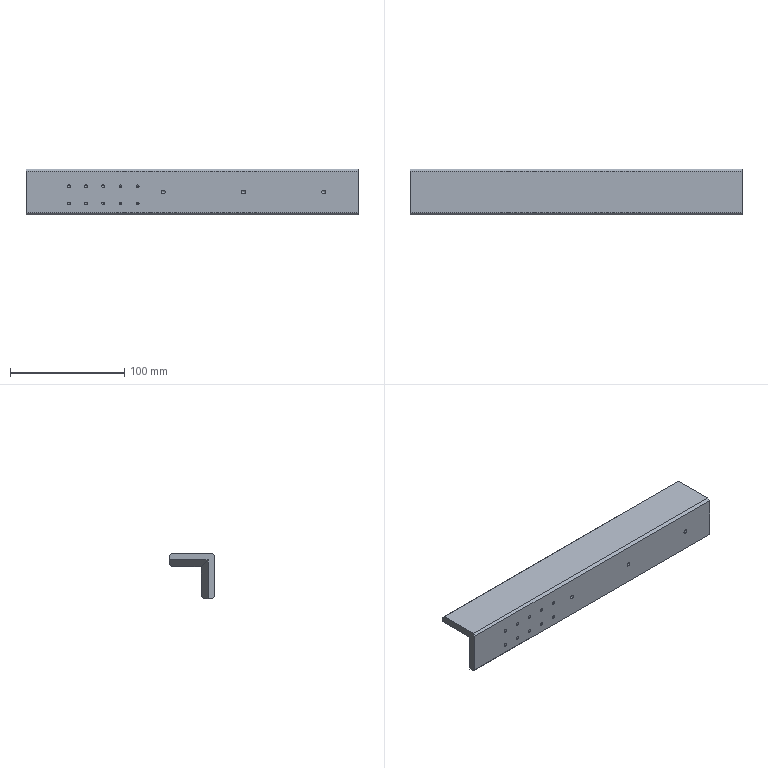Part | NX | 1 solid | 49 faces | box 290 x 40 x 40 mm | volume 230473 mm3 | cylinder 17 | cone 17 | plane 15 | commonest cylinder face diameters 2.5 x10 4.2 x4 3.3 x3
STEP:
#1=CARTESIAN_POINT('',(145.,-18.,20.));
#2=VERTEX_POINT('',#1);
#3=CARTESIAN_POINT('',(145.,-20.,18.));
#4=VERTEX_POINT('',#3);
#5=CARTESIAN_POINT('',(145.,-19.,19.));
#6=DIRECTION('',(0.,-0.7071,-0.7071));
#7=VECTOR('',#6,1000.);
#8=LINE('',#5,#7);
#9=EDGE_CURVE('',#2,#4,#8,.T.);
#10=ORIENTED_EDGE('',*,*,#9,.F.);
#11=CARTESIAN_POINT('',(-145.,-18.,20.));
#12=VERTEX_POINT('',#11);
#13=CARTESIAN_POINT('',(145.,-18.,20.));
#14=DIRECTION('',(1.,0.,0.));
#15=VECTOR('',#14,1000.);
#16=LINE('',#13,#15);
#17=EDGE_CURVE('',#12,#2,#16,.T.);
#18=ORIENTED_EDGE('',*,*,#17,.F.);
#19=CARTESIAN_POINT('',(-145.,-20.,18.));
#20=VERTEX_POINT('',#19);
#21=CARTESIAN_POINT('',(-145.,-20.,18.));
#22=DIRECTION('',(0.,0.7071,0.7071));
#23=VECTOR('',#22,1000.);
#24=LINE('',#21,#23);
#25=EDGE_CURVE('',#20,#12,#24,.T.);
#26=ORIENTED_EDGE('',*,*,#25,.F.);
#27=CARTESIAN_POINT('',(145.,-20.,18.));
#28=DIRECTION('',(-1.,0.,0.));
#29=VECTOR('',#28,1000.);
#30=LINE('',#27,#29);
#31=EDGE_CURVE('',#4,#20,#30,.T.);
#32=ORIENTED_EDGE('',*,*,#31,.F.);
#33=EDGE_LOOP('',(#10,#18,#26,#32));
#34=FACE_BOUND('',#33,.T.);
#35=CARTESIAN_POINT('',(145.,-20.,18.));
#36=DIRECTION('',(0.,0.7071,-0.7071));
#37=DIRECTION('',(-1.,0.,0.));
#38=AXIS2_PLACEMENT_3D('',#35,#36,#37);
#39=PLANE('',#38);
#40=ADVANCED_FACE('',(#34),#39,.F.);
#41=CARTESIAN_POINT('',(145.,-20.,-18.));
#42=VERTEX_POINT('',#41);
#43=CARTESIAN_POINT('',(145.,-18.,-20.));
#44=VERTEX_POINT('',#43);
#45=CARTESIAN_POINT('',(145.,-19.,-19.));
#46=DIRECTION('',(0.,0.7071,-0.7071));
#47=VECTOR('',#46,1000.);
#48=LINE('',#45,#47);
#49=EDGE_CURVE('',#42,#44,#48,.T.);
#50=ORIENTED_EDGE('',*,*,#49,.F.);
#51=CARTESIAN_POINT('',(-145.,-20.,-18.));
#52=VERTEX_POINT('',#51);
#53=CARTESIAN_POINT('',(145.,-20.,-18.));
#54=DIRECTION('',(1.,0.,0.));
#55=VECTOR('',#54,1000.);
#56=LINE('',#53,#55);
#57=EDGE_CURVE('',#52,#42,#56,.T.);
#58=ORIENTED_EDGE('',*,*,#57,.F.);
#59=CARTESIAN_POINT('',(-145.,-18.,-20.));
#60=VERTEX_POINT('',#59);
#61=CARTESIAN_POINT('',(-145.,-18.,-20.));
#62=DIRECTION('',(0.,-0.7071,0.7071));
#63=VECTOR('',#62,1000.);
#64=LINE('',#61,#63);
#65=EDGE_CURVE('',#60,#52,#64,.T.);
#66=ORIENTED_EDGE('',*,*,#65,.F.);
#67=CARTESIAN_POINT('',(145.,-18.,-20.));
#68=DIRECTION('',(-1.,0.,0.));
#69=VECTOR('',#68,1000.);
#70=LINE('',#67,#69);
#71=EDGE_CURVE('',#44,#60,#70,.T.);
#72=ORIENTED_EDGE('',*,*,#71,.F.);
#73=EDGE_LOOP('',(#50,#58,#66,#72));
#74=FACE_BOUND('',#73,.T.);
#75=CARTESIAN_POINT('',(145.,-18.,-20.));
#76=DIRECTION('',(0.,0.7071,0.7071));
#77=DIRECTION('',(-1.,0.,0.));
#78=AXIS2_PLACEMENT_3D('',#75,#76,#77);
#79=PLANE('',#78);
#80=ADVANCED_FACE('',(#74),#79,.F.);
#81=CARTESIAN_POINT('',(145.,20.,18.));
#82=VERTEX_POINT('',#81);
#83=CARTESIAN_POINT('',(145.,18.,20.));
#84=VERTEX_POINT('',#83);
#85=CARTESIAN_POINT('',(145.,19.,19.));
#86=DIRECTION('',(0.,-0.7071,0.7071));
#87=VECTOR('',#86,1000.);
#88=LINE('',#85,#87);
#89=EDGE_CURVE('',#82,#84,#88,.T.);
#90=ORIENTED_EDGE('',*,*,#89,.F.);
#91=CARTESIAN_POINT('',(-145.,20.,18.));
#92=VERTEX_POINT('',#91);
#93=CARTESIAN_POINT('',(145.,20.,18.));
#94=DIRECTION('',(1.,0.,0.));
#95=VECTOR('',#94,1000.);
#96=LINE('',#93,#95);
#97=EDGE_CURVE('',#92,#82,#96,.T.);
#98=ORIENTED_EDGE('',*,*,#97,.F.);
#99=CARTESIAN_POINT('',(-145.,18.,20.));
#100=VERTEX_POINT('',#99);
#101=CARTESIAN_POINT('',(-145.,18.,20.));
#102=DIRECTION('',(0.,0.7071,-0.7071));
#103=VECTOR('',#102,1000.);
#104=LINE('',#101,#103);
#105=EDGE_CURVE('',#100,#92,#104,.T.);
#106=ORIENTED_EDGE('',*,*,#105,.F.);
#107=CARTESIAN_POINT('',(145.,18.,20.));
#108=DIRECTION('',(-1.,0.,0.));
#109=VECTOR('',#108,1000.);
#110=LINE('',#107,#109);
#111=EDGE_CURVE('',#84,#100,#110,.T.);
#112=ORIENTED_EDGE('',*,*,#111,.F.);
#113=EDGE_LOOP('',(#90,#98,#106,#112));
#114=FACE_BOUND('',#113,.T.);
#115=CARTESIAN_POINT('',(145.,18.,20.));
#116=DIRECTION('',(0.,-0.7071,-0.7071));
#117=DIRECTION('',(-1.,0.,0.));
#118=AXIS2_PLACEMENT_3D('',#115,#116,#117);
#119=PLANE('',#118);
#120=ADVANCED_FACE('',(#114),#119,.F.);
#121=CARTESIAN_POINT('',(-138.333,20.,10.));
#122=VERTEX_POINT('',#121);
#123=CARTESIAN_POINT('',(-135.,18.,8.));
#124=VERTEX_POINT('',#123);
#125=CARTESIAN_POINT('',(-136.628,18.977,8.977));
#126=DIRECTION('',(0.7625,-0.4575,-0.4575));
#127=VECTOR('',#126,1000.);
#128=LINE('',#125,#127);
#129=EDGE_CURVE('',#122,#124,#128,.T.);
#130=ORIENTED_EDGE('',*,*,#129,.F.);
#131=CARTESIAN_POINT('',(145.,20.,10.));
#132=VERTEX_POINT('',#131);
#133=CARTESIAN_POINT('',(145.,20.,10.));
#134=DIRECTION('',(-1.,0.,0.));
#135=VECTOR('',#134,1000.);
#136=LINE('',#133,#135);
#137=EDGE_CURVE('',#132,#122,#136,.T.);
#138=ORIENTED_EDGE('',*,*,#137,.F.);
#139=CARTESIAN_POINT('',(145.,18.,8.));
#140=VERTEX_POINT('',#139);
#141=CARTESIAN_POINT('',(145.,5.,-5.));
#142=DIRECTION('',(0.,0.7071,0.7071));
#143=VECTOR('',#142,1000.);
#144=LINE('',#141,#143);
#145=EDGE_CURVE('',#140,#132,#144,.T.);
#146=ORIENTED_EDGE('',*,*,#145,.F.);
#147=CARTESIAN_POINT('',(-145.,18.,8.));
#148=DIRECTION('',(1.,0.,0.));
#149=VECTOR('',#148,1000.);
#150=LINE('',#147,#149);
#151=EDGE_CURVE('',#124,#140,#150,.T.);
#152=ORIENTED_EDGE('',*,*,#151,.F.);
#153=EDGE_LOOP('',(#130,#138,#146,#152));
#154=FACE_BOUND('',#153,.T.);
#155=CARTESIAN_POINT('',(145.,-10.,-20.));
#156=DIRECTION('',(0.,-0.7071,0.7071));
#157=DIRECTION('',(1.,0.,0.));
#158=AXIS2_PLACEMENT_3D('',#155,#156,#157);
#159=PLANE('',#158);
#160=ADVANCED_FACE('',(#154),#159,.F.);
#161=CARTESIAN_POINT('',(-135.,-8.,-18.));
#162=VERTEX_POINT('',#161);
#163=CARTESIAN_POINT('',(-138.333,-10.,-20.));
#164=VERTEX_POINT('',#163);
#165=CARTESIAN_POINT('',(-136.628,-8.977,-18.977));
#166=DIRECTION('',(-0.7625,-0.4575,-0.4575));
#167=VECTOR('',#166,1000.);
#168=LINE('',#165,#167);
#169=EDGE_CURVE('',#162,#164,#168,.T.);
#170=ORIENTED_EDGE('',*,*,#169,.F.);
#171=CARTESIAN_POINT('',(145.,-8.,-18.));
#172=VERTEX_POINT('',#171);
#173=CARTESIAN_POINT('',(-145.,-8.,-18.));
#174=DIRECTION('',(-1.,0.,0.));
#175=VECTOR('',#174,1000.);
#176=LINE('',#173,#175);
#177=EDGE_CURVE('',#172,#162,#176,.T.);
#178=ORIENTED_EDGE('',*,*,#177,.F.);
#179=CARTESIAN_POINT('',(145.,-10.,-20.));
#180=VERTEX_POINT('',#179);
#181=CARTESIAN_POINT('',(145.,5.,-5.));
#182=DIRECTION('',(0.,0.7071,0.7071));
#183=VECTOR('',#182,1000.);
#184=LINE('',#181,#183);
#185=EDGE_CURVE('',#180,#172,#184,.T.);
#186=ORIENTED_EDGE('',*,*,#185,.F.);
#187=CARTESIAN_POINT('',(145.,-10.,-20.));
#188=DIRECTION('',(1.,0.,0.));
#189=VECTOR('',#188,1000.);
#190=LINE('',#187,#189);
#191=EDGE_CURVE('',#164,#180,#190,.T.);
#192=ORIENTED_EDGE('',*,*,#191,.F.);
#193=EDGE_LOOP('',(#170,#178,#186,#192));
#194=FACE_BOUND('',#193,.T.);
#195=CARTESIAN_POINT('',(145.,-10.,-20.));
#196=DIRECTION('',(0.,-0.7071,0.7071));
#197=DIRECTION('',(1.,0.,0.));
#198=AXIS2_PLACEMENT_3D('',#195,#196,#197);
#199=PLANE('',#198);
#200=ADVANCED_FACE('',(#194),#199,.F.);
#201=CARTESIAN_POINT('',(-135.,-8.,8.));
#202=VERTEX_POINT('',#201);
#203=CARTESIAN_POINT('',(-135.,-8.,-20.));
#204=DIRECTION('',(0.,0.,1.));
#205=VECTOR('',#204,1000.);
#206=LINE('',#203,#205);
#207=EDGE_CURVE('',#162,#202,#206,.T.);
#208=ORIENTED_EDGE('',*,*,#207,.F.);
#209=ORIENTED_EDGE('',*,*,#169,.T.);
#210=CARTESIAN_POINT('',(-145.,-14.,-20.));
#211=VERTEX_POINT('',#210);
#212=CARTESIAN_POINT('',(-145.,-14.,-20.));
#213=DIRECTION('',(0.8575,0.5145,0.));
#214=VECTOR('',#213,1000.);
#215=LINE('',#212,#214);
#216=EDGE_CURVE('',#211,#164,#215,.T.);
#217=ORIENTED_EDGE('',*,*,#216,.F.);
#218=CARTESIAN_POINT('',(-145.,-14.,14.));
#219=VERTEX_POINT('',#218);
#220=CARTESIAN_POINT('',(-145.,-14.,0.));
#221=DIRECTION('',(0.,0.,-1.));
#222=VECTOR('',#221,1000.);
#223=LINE('',#220,#222);
#224=EDGE_CURVE('',#219,#211,#223,.T.);
#225=ORIENTED_EDGE('',*,*,#224,.F.);
#226=CARTESIAN_POINT('',(-140.116,-11.07,11.07));
#227=DIRECTION('',(0.7625,0.4575,-0.4575));
#228=VECTOR('',#227,1000.);
#229=LINE('',#226,#228);
#230=EDGE_CURVE('',#219,#202,#229,.T.);
#231=ORIENTED_EDGE('',*,*,#230,.T.);
#232=EDGE_LOOP('',(#208,#209,#217,#225,#231));
#233=FACE_BOUND('',#232,.T.);
#234=CARTESIAN_POINT('',(-145.,-14.,0.));
#235=DIRECTION('',(0.5145,-0.8575,0.));
#236=DIRECTION('',(0.,0.,-1.));
#237=AXIS2_PLACEMENT_3D('',#234,#235,#236);
#238=PLANE('',#237);
#239=ADVANCED_FACE('',(#233),#238,.F.);
#240=CARTESIAN_POINT('',(-145.,20.,14.));
#241=VERTEX_POINT('',#240);
#242=CARTESIAN_POINT('',(-145.,20.,14.));
#243=DIRECTION('',(-0.8575,0.,0.5145));
#244=VECTOR('',#243,1000.);
#245=LINE('',#242,#244);
#246=EDGE_CURVE('',#122,#241,#245,.T.);
#247=ORIENTED_EDGE('',*,*,#246,.F.);
#248=ORIENTED_EDGE('',*,*,#129,.T.);
#249=CARTESIAN_POINT('',(-135.,20.,8.));
#250=DIRECTION('',(0.,1.,0.));
#251=VECTOR('',#250,1000.);
#252=LINE('',#249,#251);
#253=EDGE_CURVE('',#202,#124,#252,.T.);
#254=ORIENTED_EDGE('',*,*,#253,.F.);
#255=ORIENTED_EDGE('',*,*,#230,.F.);
#256=CARTESIAN_POINT('',(-145.,0.,14.));
#257=DIRECTION('',(0.,-1.,0.));
#258=VECTOR('',#257,1000.);
#259=LINE('',#256,#258);
#260=EDGE_CURVE('',#241,#219,#259,.T.);
#261=ORIENTED_EDGE('',*,*,#260,.F.);
#262=EDGE_LOOP('',(#247,#248,#254,#255,#261));
#263=FACE_BOUND('',#262,.T.);
#264=CARTESIAN_POINT('',(-145.,0.,14.));
#265=DIRECTION('',(0.5145,0.,0.8575));
#266=DIRECTION('',(0.,-1.,0.));
#267=AXIS2_PLACEMENT_3D('',#264,#265,#266);
#268=PLANE('',#267);
#269=ADVANCED_FACE('',(#263),#268,.F.);
#270=ORIENTED_EDGE('',*,*,#253,.T.);
#271=ORIENTED_EDGE('',*,*,#151,.T.);
#272=CARTESIAN_POINT('',(145.,-8.,8.));
#273=VERTEX_POINT('',#272);
#274=CARTESIAN_POINT('',(145.,20.,8.));
#275=DIRECTION('',(0.,-1.,0.));
#276=VECTOR('',#275,1000.);
#277=LINE('',#274,#276);
#278=EDGE_CURVE('',#140,#273,#277,.T.);
#279=ORIENTED_EDGE('',*,*,#278,.T.);
#280=CARTESIAN_POINT('',(-145.,-8.,8.));
#281=DIRECTION('',(1.,0.,0.));
#282=VECTOR('',#281,1000.);
#283=LINE('',#280,#282);
#284=EDGE_CURVE('',#202,#273,#283,.T.);
#285=ORIENTED_EDGE('',*,*,#284,.F.);
#286=EDGE_LOOP('',(#270,#271,#279,#285));
#287=FACE_BOUND('',#286,.T.);
#288=CARTESIAN_POINT('',(-145.,20.,8.));
#289=DIRECTION('',(0.,0.,1.));
#290=DIRECTION('',(0.,-1.,0.));
#291=AXIS2_PLACEMENT_3D('',#288,#289,#290);
#292=PLANE('',#291);
#293=ADVANCED_FACE('',(#287),#292,.F.);
#294=CARTESIAN_POINT('',(145.,-8.,-20.));
#295=DIRECTION('',(0.,0.,-1.));
#296=VECTOR('',#295,1000.);
#297=LINE('',#294,#296);
#298=EDGE_CURVE('',#273,#172,#297,.T.);
#299=ORIENTED_EDGE('',*,*,#298,.T.);
#300=ORIENTED_EDGE('',*,*,#177,.T.);
#301=ORIENTED_EDGE('',*,*,#207,.T.);
#302=ORIENTED_EDGE('',*,*,#284,.T.);
#303=EDGE_LOOP('',(#299,#300,#301,#302));
#304=FACE_BOUND('',#303,.T.);
#305=CARTESIAN_POINT('',(-145.,-8.,-20.));
#306=DIRECTION('',(0.,-1.,0.));
#307=DIRECTION('',(0.,0.,-1.));
#308=AXIS2_PLACEMENT_3D('',#305,#306,#307);
#309=PLANE('',#308);
#310=ADVANCED_FACE('',(#304),#309,.F.);
#311=CARTESIAN_POINT('',(-145.,20.,20.));
#312=DIRECTION('',(0.,-1.,0.));
#313=VECTOR('',#312,1000.);
#314=LINE('',#311,#313);
#315=EDGE_CURVE('',#100,#12,#314,.T.);
#316=ORIENTED_EDGE('',*,*,#315,.F.);
#317=ORIENTED_EDGE('',*,*,#105,.T.);
#318=CARTESIAN_POINT('',(-145.,20.,20.));
#319=DIRECTION('',(0.,0.,1.));
#320=VECTOR('',#319,1000.);
#321=LINE('',#318,#320);
#322=EDGE_CURVE('',#241,#92,#321,.T.);
#323=ORIENTED_EDGE('',*,*,#322,.F.);
#324=ORIENTED_EDGE('',*,*,#260,.T.);
#325=ORIENTED_EDGE('',*,*,#224,.T.);
#326=CARTESIAN_POINT('',(-145.,20.,-20.));
#327=DIRECTION('',(0.,1.,0.));
#328=VECTOR('',#327,1000.);
#329=LINE('',#326,#328);
#330=EDGE_CURVE('',#60,#211,#329,.T.);
#331=ORIENTED_EDGE('',*,*,#330,.F.);
#332=ORIENTED_EDGE('',*,*,#65,.T.);
#333=CARTESIAN_POINT('',(-145.,-20.,20.));
#334=DIRECTION('',(0.,0.,-1.));
#335=VECTOR('',#334,1000.);
#336=LINE('',#333,#335);
#337=EDGE_CURVE('',#20,#52,#336,.T.);
#338=ORIENTED_EDGE('',*,*,#337,.F.);
#339=ORIENTED_EDGE('',*,*,#25,.T.);
#340=EDGE_LOOP('',(#316,#317,#323,#324,#325,#331,#332,#338,#339));
#341=FACE_BOUND('',#340,.T.);
#342=CARTESIAN_POINT('',(-145.,0.,0.));
#343=DIRECTION('',(1.,0.,0.));
#344=DIRECTION('',(0.,0.,-1.));
#345=AXIS2_PLACEMENT_3D('',#342,#343,#344);
#346=PLANE('',#345);
#347=ADVANCED_FACE('',(#341),#346,.F.);
#348=CARTESIAN_POINT('',(145.,20.,-20.));
#349=DIRECTION('',(0.,1.,0.));
#350=VECTOR('',#349,1000.);
#351=LINE('',#348,#350);
#352=EDGE_CURVE('',#44,#180,#351,.T.);
#353=ORIENTED_EDGE('',*,*,#352,.T.);
#354=ORIENTED_EDGE('',*,*,#185,.T.);
#355=ORIENTED_EDGE('',*,*,#298,.F.);
#356=ORIENTED_EDGE('',*,*,#278,.F.);
#357=ORIENTED_EDGE('',*,*,#145,.T.);
#358=CARTESIAN_POINT('',(145.,20.,20.));
#359=DIRECTION('',(0.,0.,1.));
#360=VECTOR('',#359,1000.);
#361=LINE('',#358,#360);
#362=EDGE_CURVE('',#132,#82,#361,.T.);
#363=ORIENTED_EDGE('',*,*,#362,.T.);
#364=ORIENTED_EDGE('',*,*,#89,.T.);
#365=CARTESIAN_POINT('',(145.,20.,20.));
#366=DIRECTION('',(0.,-1.,0.));
#367=VECTOR('',#366,1000.);
#368=LINE('',#365,#367);
#369=EDGE_CURVE('',#84,#2,#368,.T.);
#370=ORIENTED_EDGE('',*,*,#369,.T.);
#371=ORIENTED_EDGE('',*,*,#9,.T.);
#372=CARTESIAN_POINT('',(145.,-20.,20.));
#373=DIRECTION('',(0.,0.,-1.));
#374=VECTOR('',#373,1000.);
#375=LINE('',#372,#374);
#376=EDGE_CURVE('',#4,#42,#375,.T.);
#377=ORIENTED_EDGE('',*,*,#376,.T.);
#378=ORIENTED_EDGE('',*,*,#49,.T.);
#379=EDGE_LOOP('',(#353,#354,#355,#356,#357,#363,#364,#370,#371,#377,#378));
#380=FACE_BOUND('',#379,.T.);
#381=CARTESIAN_POINT('',(145.,14.,11.9));
#382=VERTEX_POINT('',#381);
#383=CARTESIAN_POINT('',(145.,14.,14.));
#384=DIRECTION('',(1.,0.,0.));
#385=DIRECTION('',(0.,0.,-1.));
#386=AXIS2_PLACEMENT_3D('',#383,#384,#385);
#387=CIRCLE('',#386,2.1);
#388=EDGE_CURVE('',#382,#382,#387,.T.);
#389=ORIENTED_EDGE('',*,*,#388,.F.);
#390=EDGE_LOOP('',(#389));
#391=FACE_BOUND('',#390,.T.);
#392=CARTESIAN_POINT('',(145.,-2.,11.9));
#393=VERTEX_POINT('',#392);
#394=CARTESIAN_POINT('',(145.,-2.,14.));
#395=DIRECTION('',(1.,0.,0.));
#396=DIRECTION('',(0.,0.,-1.));
#397=AXIS2_PLACEMENT_3D('',#394,#395,#396);
#398=CIRCLE('',#397,2.1);
#399=EDGE_CURVE('',#393,#393,#398,.T.);
#400=ORIENTED_EDGE('',*,*,#399,.F.);
#401=EDGE_LOOP('',(#400));
#402=FACE_BOUND('',#401,.T.);
#403=CARTESIAN_POINT('',(145.,-14.,-0.1));
#404=VERTEX_POINT('',#403);
#405=CARTESIAN_POINT('',(145.,-14.,2.));
#406=DIRECTION('',(1.,0.,0.));
#407=DIRECTION('',(0.,0.,-1.));
#408=AXIS2_PLACEMENT_3D('',#405,#406,#407);
#409=CIRCLE('',#408,2.1);
#410=EDGE_CURVE('',#404,#404,#409,.T.);
#411=ORIENTED_EDGE('',*,*,#410,.F.);
#412=EDGE_LOOP('',(#411));
#413=FACE_BOUND('',#412,.T.);
#414=CARTESIAN_POINT('',(145.,-14.,-16.1));
#415=VERTEX_POINT('',#414);
#416=CARTESIAN_POINT('',(145.,-14.,-14.));
#417=DIRECTION('',(1.,0.,0.));
#418=DIRECTION('',(0.,0.,-1.));
#419=AXIS2_PLACEMENT_3D('',#416,#417,#418);
#420=CIRCLE('',#419,2.1);
#421=EDGE_CURVE('',#415,#415,#420,.T.);
#422=ORIENTED_EDGE('',*,*,#421,.F.);
#423=EDGE_LOOP('',(#422));
#424=FACE_BOUND('',#423,.T.);
#425=CARTESIAN_POINT('',(145.,0.,0.));
#426=DIRECTION('',(1.,0.,0.));
#427=DIRECTION('',(0.,0.,-1.));
#428=AXIS2_PLACEMENT_3D('',#425,#426,#427);
#429=PLANE('',#428);
#430=ADVANCED_FACE('',(#380,#391,#402,#413,#424),#429,.T.);
#431=CARTESIAN_POINT('',(-107.5,-20.,3.75));
#432=VERTEX_POINT('',#431);
#433=CARTESIAN_POINT('',(-107.5,-20.,5.));
#434=DIRECTION('',(0.,-1.,0.));
#435=DIRECTION('',(0.,0.,-1.));
#436=AXIS2_PLACEMENT_3D('',#433,#434,#435);
#437=CIRCLE('',#436,1.25);
#438=EDGE_CURVE('',#432,#432,#437,.T.);
#439=ORIENTED_EDGE('',*,*,#438,.F.);
#440=EDGE_LOOP('',(#439));
#441=FACE_BOUND('',#440,.T.);
#442=CARTESIAN_POINT('',(-92.5,-20.,3.75));
#443=VERTEX_POINT('',#442);
#444=CARTESIAN_POINT('',(-92.5,-20.,5.));
#445=DIRECTION('',(0.,-1.,0.));
#446=DIRECTION('',(0.,0.,-1.));
#447=AXIS2_PLACEMENT_3D('',#444,#445,#446);
#448=CIRCLE('',#447,1.25);
#449=EDGE_CURVE('',#443,#443,#448,.T.);
#450=ORIENTED_EDGE('',*,*,#449,.F.);
#451=EDGE_LOOP('',(#450));
#452=FACE_BOUND('',#451,.T.);
#453=CARTESIAN_POINT('',(-77.5,-20.,3.75));
#454=VERTEX_POINT('',#453);
#455=CARTESIAN_POINT('',(-77.5,-20.,5.));
#456=DIRECTION('',(0.,-1.,0.));
#457=DIRECTION('',(0.,0.,-1.));
#458=AXIS2_PLACEMENT_3D('',#455,#456,#457);
#459=CIRCLE('',#458,1.25);
#460=EDGE_CURVE('',#454,#454,#459,.T.);
#461=ORIENTED_EDGE('',*,*,#460,.F.);
#462=EDGE_LOOP('',(#461));
#463=FACE_BOUND('',#462,.T.);
#464=CARTESIAN_POINT('',(-107.5,-20.,-11.25));
#465=VERTEX_POINT('',#464);
#466=CARTESIAN_POINT('',(-107.5,-20.,-10.));
#467=DIRECTION('',(0.,-1.,0.));
#468=DIRECTION('',(0.,0.,-1.));
#469=AXIS2_PLACEMENT_3D('',#466,#467,#468);
#470=CIRCLE('',#469,1.25);
#471=EDGE_CURVE('',#465,#465,#470,.T.);
#472=ORIENTED_EDGE('',*,*,#471,.F.);
#473=EDGE_LOOP('',(#472));
#474=FACE_BOUND('',#473,.T.);
#475=CARTESIAN_POINT('',(-92.5,-20.,-11.25));
#476=VERTEX_POINT('',#475);
#477=CARTESIAN_POINT('',(-92.5,-20.,-10.));
#478=DIRECTION('',(0.,-1.,0.));
#479=DIRECTION('',(0.,0.,-1.));
#480=AXIS2_PLACEMENT_3D('',#477,#478,#479);
#481=CIRCLE('',#480,1.25);
#482=EDGE_CURVE('',#476,#476,#481,.T.);
#483=ORIENTED_EDGE('',*,*,#482,.F.);
#484=EDGE_LOOP('',(#483));
#485=FACE_BOUND('',#484,.T.);
#486=CARTESIAN_POINT('',(-77.5,-20.,-11.25));
#487=VERTEX_POINT('',#486);
#488=CARTESIAN_POINT('',(-77.5,-20.,-10.));
#489=DIRECTION('',(0.,-1.,0.));
#490=DIRECTION('',(0.,0.,-1.));
#491=AXIS2_PLACEMENT_3D('',#488,#489,#490);
#492=CIRCLE('',#491,1.25);
#493=EDGE_CURVE('',#487,#487,#492,.T.);
#494=ORIENTED_EDGE('',*,*,#493,.F.);
#495=EDGE_LOOP('',(#494));
#496=FACE_BOUND('',#495,.T.);
#497=ORIENTED_EDGE('',*,*,#337,.T.);
#498=ORIENTED_EDGE('',*,*,#57,.T.);
#499=ORIENTED_EDGE('',*,*,#376,.F.);
#500=ORIENTED_EDGE('',*,*,#31,.T.);
#501=EDGE_LOOP('',(#497,#498,#499,#500));
#502=FACE_BOUND('',#501,.T.);
#503=CARTESIAN_POINT('',(-47.5,-20.,3.75));
#504=VERTEX_POINT('',#503);
#505=CARTESIAN_POINT('',(-47.5,-20.,5.));
#506=DIRECTION('',(0.,-1.,0.));
#507=DIRECTION('',(0.,0.,-1.));
#508=AXIS2_PLACEMENT_3D('',#505,#506,#507);
#509=CIRCLE('',#508,1.25);
#510=EDGE_CURVE('',#504,#504,#509,.T.);
#511=ORIENTED_EDGE('',*,*,#510,.F.);
#512=EDGE_LOOP('',(#511));
#513=FACE_BOUND('',#512,.T.);
#514=CARTESIAN_POINT('',(-47.5,-20.,-11.25));
#515=VERTEX_POINT('',#514);
#516=CARTESIAN_POINT('',(-47.5,-20.,-10.));
#517=DIRECTION('',(0.,-1.,0.));
#518=DIRECTION('',(0.,0.,-1.));
#519=AXIS2_PLACEMENT_3D('',#516,#517,#518);
#520=CIRCLE('',#519,1.25);
#521=EDGE_CURVE('',#515,#515,#520,.T.);
#522=ORIENTED_EDGE('',*,*,#521,.F.);
#523=EDGE_LOOP('',(#522));
#524=FACE_BOUND('',#523,.T.);
#525=CARTESIAN_POINT('',(-62.5,-20.,-11.25));
#526=VERTEX_POINT('',#525);
#527=CARTESIAN_POINT('',(-62.5,-20.,-10.));
#528=DIRECTION('',(0.,-1.,0.));
#529=DIRECTION('',(0.,0.,-1.));
#530=AXIS2_PLACEMENT_3D('',#527,#528,#529);
#531=CIRCLE('',#530,1.25);
#532=EDGE_CURVE('',#526,#526,#531,.T.);
#533=ORIENTED_EDGE('',*,*,#532,.F.);
#534=EDGE_LOOP('',(#533));
#535=FACE_BOUND('',#534,.T.);
#536=CARTESIAN_POINT('',(-62.5,-20.,3.75));
#537=VERTEX_POINT('',#536);
#538=CARTESIAN_POINT('',(-62.5,-20.,5.));
#539=DIRECTION('',(0.,-1.,0.));
#540=DIRECTION('',(0.,0.,-1.));
#541=AXIS2_PLACEMENT_3D('',#538,#539,#540);
#542=CIRCLE('',#541,1.25);
#543=EDGE_CURVE('',#537,#537,#542,.T.);
#544=ORIENTED_EDGE('',*,*,#543,.F.);
#545=EDGE_LOOP('',(#544));
#546=FACE_BOUND('',#545,.T.);
#547=CARTESIAN_POINT('',(115.,-20.,-1.65));
#548=VERTEX_POINT('',#547);
#549=CARTESIAN_POINT('',(115.,-20.,0.));
#550=DIRECTION('',(0.,-1.,0.));
#551=DIRECTION('',(0.,0.,-1.));
#552=AXIS2_PLACEMENT_3D('',#549,#550,#551);
#553=CIRCLE('',#552,1.65);
#554=EDGE_CURVE('',#548,#548,#553,.T.);
#555=ORIENTED_EDGE('',*,*,#554,.F.);
#556=EDGE_LOOP('',(#555));
#557=FACE_BOUND('',#556,.T.);
#558=CARTESIAN_POINT('',(45.,-20.,-1.65));
#559=VERTEX_POINT('',#558);
#560=CARTESIAN_POINT('',(45.,-20.,0.));
#561=DIRECTION('',(0.,-1.,0.));
#562=DIRECTION('',(0.,0.,-1.));
#563=AXIS2_PLACEMENT_3D('',#560,#561,#562);
#564=CIRCLE('',#563,1.65);
#565=EDGE_CURVE('',#559,#559,#564,.T.);
#566=ORIENTED_EDGE('',*,*,#565,.F.);
#567=EDGE_LOOP('',(#566));
#568=FACE_BOUND('',#567,.T.);
#569=CARTESIAN_POINT('',(-25.,-20.,-1.65));
#570=VERTEX_POINT('',#569);
#571=CARTESIAN_POINT('',(-25.,-20.,0.));
#572=DIRECTION('',(0.,-1.,0.));
#573=DIRECTION('',(0.,0.,-1.));
#574=AXIS2_PLACEMENT_3D('',#571,#572,#573);
#575=CIRCLE('',#574,1.65);
#576=EDGE_CURVE('',#570,#570,#575,.T.);
#577=ORIENTED_EDGE('',*,*,#576,.F.);
#578=EDGE_LOOP('',(#577));
#579=FACE_BOUND('',#578,.T.);
#580=CARTESIAN_POINT('',(145.,-20.,20.));
#581=DIRECTION('',(0.,1.,0.));
#582=DIRECTION('',(0.,0.,1.));
#583=AXIS2_PLACEMENT_3D('',#580,#581,#582);
#584=PLANE('',#583);
#585=ADVANCED_FACE('',(#441,#452,#463,#474,#485,#496,#502,#513,#524,#535,#546,#557,#568,#579),#584,.F.);
#586=ORIENTED_EDGE('',*,*,#369,.F.);
#587=ORIENTED_EDGE('',*,*,#111,.T.);
#588=ORIENTED_EDGE('',*,*,#315,.T.);
#589=ORIENTED_EDGE('',*,*,#17,.T.);
#590=EDGE_LOOP('',(#586,#587,#588,#589));
#591=FACE_BOUND('',#590,.T.);
#592=CARTESIAN_POINT('',(145.,20.,20.));
#593=DIRECTION('',(0.,0.,-1.));
#594=DIRECTION('',(0.,1.,0.));
#595=AXIS2_PLACEMENT_3D('',#592,#593,#594);
#596=PLANE('',#595);
#597=ADVANCED_FACE('',(#591),#596,.F.);
#598=ORIENTED_EDGE('',*,*,#362,.F.);
#599=ORIENTED_EDGE('',*,*,#137,.T.);
#600=ORIENTED_EDGE('',*,*,#246,.T.);
#601=ORIENTED_EDGE('',*,*,#322,.T.);
#602=ORIENTED_EDGE('',*,*,#97,.T.);
#603=EDGE_LOOP('',(#598,#599,#600,#601,#602));
#604=FACE_BOUND('',#603,.T.);
#605=CARTESIAN_POINT('',(145.,20.,20.));
#606=DIRECTION('',(0.,-1.,0.));
#607=DIRECTION('',(0.,0.,-1.));
#608=AXIS2_PLACEMENT_3D('',#605,#606,#607);
#609=PLANE('',#608);
#610=ADVANCED_FACE('',(#604),#609,.F.);
#611=ORIENTED_EDGE('',*,*,#216,.T.);
#612=ORIENTED_EDGE('',*,*,#191,.T.);
#613=ORIENTED_EDGE('',*,*,#352,.F.);
#614=ORIENTED_EDGE('',*,*,#71,.T.);
#615=ORIENTED_EDGE('',*,*,#330,.T.);
#616=EDGE_LOOP('',(#611,#612,#613,#614,#615));
#617=FACE_BOUND('',#616,.T.);
#618=CARTESIAN_POINT('',(145.,20.,-20.));
#619=DIRECTION('',(0.,0.,1.));
#620=DIRECTION('',(0.,-1.,0.));
#621=AXIS2_PLACEMENT_3D('',#618,#619,#620);
#622=PLANE('',#621);
#623=ADVANCED_FACE('',(#617),#622,.F.);
#624=ORIENTED_EDGE('',*,*,#438,.T.);
#625=EDGE_LOOP('',(#624));
#626=FACE_BOUND('',#625,.T.);
#627=CARTESIAN_POINT('',(-107.5,-12.5,3.75));
#628=VERTEX_POINT('',#627);
#629=CARTESIAN_POINT('',(-107.5,-12.5,5.));
#630=DIRECTION('',(0.,-1.,0.));
#631=DIRECTION('',(0.,0.,-1.));
#632=AXIS2_PLACEMENT_3D('',#629,#630,#631);
#633=CIRCLE('',#632,1.25);
#634=EDGE_CURVE('',#628,#628,#633,.T.);
#635=ORIENTED_EDGE('',*,*,#634,.F.);
#636=EDGE_LOOP('',(#635));
#637=FACE_BOUND('',#636,.T.);
#638=CARTESIAN_POINT('',(-107.5,-20.,5.));
#639=DIRECTION('',(0.,-1.,0.));
#640=DIRECTION('',(0.,0.,-1.));
#641=AXIS2_PLACEMENT_3D('',#638,#639,#640);
#642=CYLINDRICAL_SURFACE('',#641,1.25);
#643=ADVANCED_FACE('',(#626,#637),#642,.F.);
#644=CARTESIAN_POINT('',(-107.5,-11.749,5.));
#645=VERTEX_POINT('',#644);
#646=VERTEX_LOOP('',#645);
#647=FACE_BOUND('',#646,.T.);
#648=ORIENTED_EDGE('',*,*,#634,.T.);
#649=EDGE_LOOP('',(#648));
#650=FACE_BOUND('',#649,.T.);
#651=CARTESIAN_POINT('',(-107.5,-12.5,5.));
#652=DIRECTION('',(0.,-1.,0.));
#653=DIRECTION('',(0.,0.,-1.));
#654=AXIS2_PLACEMENT_3D('',#651,#652,#653);
#655=CONICAL_SURFACE('',#654,1.25,1.03);
#656=ADVANCED_FACE('',(#647,#650),#655,.F.);
#657=ORIENTED_EDGE('',*,*,#449,.T.);
#658=EDGE_LOOP('',(#657));
#659=FACE_BOUND('',#658,.T.);
#660=CARTESIAN_POINT('',(-92.5,-12.5,3.75));
#661=VERTEX_POINT('',#660);
#662=CARTESIAN_POINT('',(-92.5,-12.5,5.));
#663=DIRECTION('',(0.,-1.,0.));
#664=DIRECTION('',(0.,0.,-1.));
#665=AXIS2_PLACEMENT_3D('',#662,#663,#664);
#666=CIRCLE('',#665,1.25);
#667=EDGE_CURVE('',#661,#661,#666,.T.);
#668=ORIENTED_EDGE('',*,*,#667,.F.);
#669=EDGE_LOOP('',(#668));
#670=FACE_BOUND('',#669,.T.);
#671=CARTESIAN_POINT('',(-92.5,-20.,5.));
#672=DIRECTION('',(0.,-1.,0.));
#673=DIRECTION('',(0.,0.,-1.));
#674=AXIS2_PLACEMENT_3D('',#671,#672,#673);
#675=CYLINDRICAL_SURFACE('',#674,1.25);
#676=ADVANCED_FACE('',(#659,#670),#675,.F.);
#677=CARTESIAN_POINT('',(-92.5,-11.749,5.));
#678=VERTEX_POINT('',#677);
#679=VERTEX_LOOP('',#678);
#680=FACE_BOUND('',#679,.T.);
#681=ORIENTED_EDGE('',*,*,#667,.T.);
#682=EDGE_LOOP('',(#681));
#683=FACE_BOUND('',#682,.T.);
#684=CARTESIAN_POINT('',(-92.5,-12.5,5.));
#685=DIRECTION('',(0.,-1.,0.));
#686=DIRECTION('',(0.,0.,-1.));
#687=AXIS2_PLACEMENT_3D('',#684,#685,#686);
#688=CONICAL_SURFACE('',#687,1.25,1.03);
#689=ADVANCED_FACE('',(#680,#683),#688,.F.);
#690=ORIENTED_EDGE('',*,*,#460,.T.);
#691=EDGE_LOOP('',(#690));
#692=FACE_BOUND('',#691,.T.);
#693=CARTESIAN_POINT('',(-77.5,-12.5,3.75));
#694=VERTEX_POINT('',#693);
#695=CARTESIAN_POINT('',(-77.5,-12.5,5.));
#696=DIRECTION('',(0.,-1.,0.));
#697=DIRECTION('',(0.,0.,-1.));
#698=AXIS2_PLACEMENT_3D('',#695,#696,#697);
#699=CIRCLE('',#698,1.25);
#700=EDGE_CURVE('',#694,#694,#699,.T.);
#701=ORIENTED_EDGE('',*,*,#700,.F.);
#702=EDGE_LOOP('',(#701));
#703=FACE_BOUND('',#702,.T.);
#704=CARTESIAN_POINT('',(-77.5,-20.,5.));
#705=DIRECTION('',(0.,-1.,0.));
#706=DIRECTION('',(0.,0.,-1.));
#707=AXIS2_PLACEMENT_3D('',#704,#705,#706);
#708=CYLINDRICAL_SURFACE('',#707,1.25);
#709=ADVANCED_FACE('',(#692,#703),#708,.F.);
#710=CARTESIAN_POINT('',(-77.5,-11.749,5.));
#711=VERTEX_POINT('',#710);
#712=VERTEX_LOOP('',#711);
#713=FACE_BOUND('',#712,.T.);
#714=ORIENTED_EDGE('',*,*,#700,.T.);
#715=EDGE_LOOP('',(#714));
#716=FACE_BOUND('',#715,.T.);
#717=CARTESIAN_POINT('',(-77.5,-12.5,5.));
#718=DIRECTION('',(0.,-1.,0.));
#719=DIRECTION('',(0.,0.,-1.));
#720=AXIS2_PLACEMENT_3D('',#717,#718,#719);
#721=CONICAL_SURFACE('',#720,1.25,1.03);
#722=ADVANCED_FACE('',(#713,#716),#721,.F.);
#723=ORIENTED_EDGE('',*,*,#471,.T.);
#724=EDGE_LOOP('',(#723));
#725=FACE_BOUND('',#724,.T.);
#726=CARTESIAN_POINT('',(-107.5,-12.5,-11.25));
#727=VERTEX_POINT('',#726);
#728=CARTESIAN_POINT('',(-107.5,-12.5,-10.));
#729=DIRECTION('',(0.,-1.,0.));
#730=DIRECTION('',(0.,0.,-1.));
#731=AXIS2_PLACEMENT_3D('',#728,#729,#730);
#732=CIRCLE('',#731,1.25);
#733=EDGE_CURVE('',#727,#727,#732,.T.);
#734=ORIENTED_EDGE('',*,*,#733,.F.);
#735=EDGE_LOOP('',(#734));
#736=FACE_BOUND('',#735,.T.);
#737=CARTESIAN_POINT('',(-107.5,-20.,-10.));
#738=DIRECTION('',(0.,-1.,0.));
#739=DIRECTION('',(0.,0.,-1.));
#740=AXIS2_PLACEMENT_3D('',#737,#738,#739);
#741=CYLINDRICAL_SURFACE('',#740,1.25);
#742=ADVANCED_FACE('',(#725,#736),#741,.F.);
#743=CARTESIAN_POINT('',(-107.5,-11.749,-10.));
#744=VERTEX_POINT('',#743);
#745=VERTEX_LOOP('',#744);
#746=FACE_BOUND('',#745,.T.);
#747=ORIENTED_EDGE('',*,*,#733,.T.);
#748=EDGE_LOOP('',(#747));
#749=FACE_BOUND('',#748,.T.);
#750=CARTESIAN_POINT('',(-107.5,-12.5,-10.));
#751=DIRECTION('',(0.,-1.,0.));
#752=DIRECTION('',(0.,0.,-1.));
#753=AXIS2_PLACEMENT_3D('',#750,#751,#752);
#754=CONICAL_SURFACE('',#753,1.25,1.03);
#755=ADVANCED_FACE('',(#746,#749),#754,.F.);
#756=ORIENTED_EDGE('',*,*,#482,.T.);
#757=EDGE_LOOP('',(#756));
#758=FACE_BOUND('',#757,.T.);
#759=CARTESIAN_POINT('',(-92.5,-12.5,-11.25));
#760=VERTEX_POINT('',#759);
#761=CARTESIAN_POINT('',(-92.5,-12.5,-10.));
#762=DIRECTION('',(0.,-1.,0.));
#763=DIRECTION('',(0.,0.,-1.));
#764=AXIS2_PLACEMENT_3D('',#761,#762,#763);
#765=CIRCLE('',#764,1.25);
#766=EDGE_CURVE('',#760,#760,#765,.T.);
#767=ORIENTED_EDGE('',*,*,#766,.F.);
#768=EDGE_LOOP('',(#767));
#769=FACE_BOUND('',#768,.T.);
#770=CARTESIAN_POINT('',(-92.5,-20.,-10.));
#771=DIRECTION('',(0.,-1.,0.));
#772=DIRECTION('',(0.,0.,-1.));
#773=AXIS2_PLACEMENT_3D('',#770,#771,#772);
#774=CYLINDRICAL_SURFACE('',#773,1.25);
#775=ADVANCED_FACE('',(#758,#769),#774,.F.);
#776=CARTESIAN_POINT('',(-92.5,-11.749,-10.));
#777=VERTEX_POINT('',#776);
#778=VERTEX_LOOP('',#777);
#779=FACE_BOUND('',#778,.T.);
#780=ORIENTED_EDGE('',*,*,#766,.T.);
#781=EDGE_LOOP('',(#780));
#782=FACE_BOUND('',#781,.T.);
#783=CARTESIAN_POINT('',(-92.5,-12.5,-10.));
#784=DIRECTION('',(0.,-1.,0.));
#785=DIRECTION('',(0.,0.,-1.));
#786=AXIS2_PLACEMENT_3D('',#783,#784,#785);
#787=CONICAL_SURFACE('',#786,1.25,1.03);
#788=ADVANCED_FACE('',(#779,#782),#787,.F.);
#789=ORIENTED_EDGE('',*,*,#493,.T.);
#790=EDGE_LOOP('',(#789));
#791=FACE_BOUND('',#790,.T.);
#792=CARTESIAN_POINT('',(-77.5,-12.5,-11.25));
#793=VERTEX_POINT('',#792);
#794=CARTESIAN_POINT('',(-77.5,-12.5,-10.));
#795=DIRECTION('',(0.,-1.,0.));
#796=DIRECTION('',(0.,0.,-1.));
#797=AXIS2_PLACEMENT_3D('',#794,#795,#796);
#798=CIRCLE('',#797,1.25);
#799=EDGE_CURVE('',#793,#793,#798,.T.);
#800=ORIENTED_EDGE('',*,*,#799,.F.);
#801=EDGE_LOOP('',(#800));
#802=FACE_BOUND('',#801,.T.);
#803=CARTESIAN_POINT('',(-77.5,-20.,-10.));
#804=DIRECTION('',(0.,-1.,0.));
#805=DIRECTION('',(0.,0.,-1.));
#806=AXIS2_PLACEMENT_3D('',#803,#804,#805);
#807=CYLINDRICAL_SURFACE('',#806,1.25);
#808=ADVANCED_FACE('',(#791,#802),#807,.F.);
#809=CARTESIAN_POINT('',(-77.5,-11.749,-10.));
#810=VERTEX_POINT('',#809);
#811=VERTEX_LOOP('',#810);
#812=FACE_BOUND('',#811,.T.);
#813=ORIENTED_EDGE('',*,*,#799,.T.);
#814=EDGE_LOOP('',(#813));
#815=FACE_BOUND('',#814,.T.);
#816=CARTESIAN_POINT('',(-77.5,-12.5,-10.));
#817=DIRECTION('',(0.,-1.,0.));
#818=DIRECTION('',(0.,0.,-1.));
#819=AXIS2_PLACEMENT_3D('',#816,#817,#818);
#820=CONICAL_SURFACE('',#819,1.25,1.03);
#821=ADVANCED_FACE('',(#812,#815),#820,.F.);
#822=CARTESIAN_POINT('',(128.738,14.,14.));
#823=VERTEX_POINT('',#822);
#824=VERTEX_LOOP('',#823);
#825=FACE_BOUND('',#824,.T.);
#826=CARTESIAN_POINT('',(130.,14.,11.9));
#827=VERTEX_POINT('',#826);
#828=CARTESIAN_POINT('',(130.,14.,14.));
#829=DIRECTION('',(1.,0.,0.));
#830=DIRECTION('',(0.,0.,-1.));
#831=AXIS2_PLACEMENT_3D('',#828,#829,#830);
#832=CIRCLE('',#831,2.1);
#833=EDGE_CURVE('',#827,#827,#832,.T.);
#834=ORIENTED_EDGE('',*,*,#833,.T.);
#835=EDGE_LOOP('',(#834));
#836=FACE_BOUND('',#835,.T.);
#837=CARTESIAN_POINT('',(130.,14.,14.));
#838=DIRECTION('',(1.,0.,0.));
#839=DIRECTION('',(0.,0.,-1.));
#840=AXIS2_PLACEMENT_3D('',#837,#838,#839);
#841=CONICAL_SURFACE('',#840,2.1,1.03);
#842=ADVANCED_FACE('',(#825,#836),#841,.F.);
#843=ORIENTED_EDGE('',*,*,#388,.T.);
#844=EDGE_LOOP('',(#843));
#845=FACE_BOUND('',#844,.T.);
#846=ORIENTED_EDGE('',*,*,#833,.F.);
#847=EDGE_LOOP('',(#846));
#848=FACE_BOUND('',#847,.T.);
#849=CARTESIAN_POINT('',(145.,14.,14.));
#850=DIRECTION('',(1.,0.,0.));
#851=DIRECTION('',(0.,0.,-1.));
#852=AXIS2_PLACEMENT_3D('',#849,#850,#851);
#853=CYLINDRICAL_SURFACE('',#852,2.1);
#854=ADVANCED_FACE('',(#845,#848),#853,.F.);
#855=CARTESIAN_POINT('',(128.738,-2.,14.));
#856=VERTEX_POINT('',#855);
#857=VERTEX_LOOP('',#856);
#858=FACE_BOUND('',#857,.T.);
#859=CARTESIAN_POINT('',(130.,-2.,11.9));
#860=VERTEX_POINT('',#859);
#861=CARTESIAN_POINT('',(130.,-2.,14.));
#862=DIRECTION('',(1.,0.,0.));
#863=DIRECTION('',(0.,0.,-1.));
#864=AXIS2_PLACEMENT_3D('',#861,#862,#863);
#865=CIRCLE('',#864,2.1);
#866=EDGE_CURVE('',#860,#860,#865,.T.);
#867=ORIENTED_EDGE('',*,*,#866,.T.);
#868=EDGE_LOOP('',(#867));
#869=FACE_BOUND('',#868,.T.);
#870=CARTESIAN_POINT('',(130.,-2.,14.));
#871=DIRECTION('',(1.,0.,0.));
#872=DIRECTION('',(0.,0.,-1.));
#873=AXIS2_PLACEMENT_3D('',#870,#871,#872);
#874=CONICAL_SURFACE('',#873,2.1,1.03);
#875=ADVANCED_FACE('',(#858,#869),#874,.F.);
#876=ORIENTED_EDGE('',*,*,#399,.T.);
#877=EDGE_LOOP('',(#876));
#878=FACE_BOUND('',#877,.T.);
#879=ORIENTED_EDGE('',*,*,#866,.F.);
#880=EDGE_LOOP('',(#879));
#881=FACE_BOUND('',#880,.T.);
#882=CARTESIAN_POINT('',(145.,-2.,14.));
#883=DIRECTION('',(1.,0.,0.));
#884=DIRECTION('',(0.,0.,-1.));
#885=AXIS2_PLACEMENT_3D('',#882,#883,#884);
#886=CYLINDRICAL_SURFACE('',#885,2.1);
#887=ADVANCED_FACE('',(#878,#881),#886,.F.);
#888=CARTESIAN_POINT('',(128.738,-14.,2.));
#889=VERTEX_POINT('',#888);
#890=VERTEX_LOOP('',#889);
#891=FACE_BOUND('',#890,.T.);
#892=CARTESIAN_POINT('',(130.,-14.,-0.1));
#893=VERTEX_POINT('',#892);
#894=CARTESIAN_POINT('',(130.,-14.,2.));
#895=DIRECTION('',(1.,0.,0.));
#896=DIRECTION('',(0.,0.,-1.));
#897=AXIS2_PLACEMENT_3D('',#894,#895,#896);
#898=CIRCLE('',#897,2.1);
#899=EDGE_CURVE('',#893,#893,#898,.T.);
#900=ORIENTED_EDGE('',*,*,#899,.T.);
#901=EDGE_LOOP('',(#900));
#902=FACE_BOUND('',#901,.T.);
#903=CARTESIAN_POINT('',(130.,-14.,2.));
#904=DIRECTION('',(1.,0.,0.));
#905=DIRECTION('',(0.,0.,-1.));
#906=AXIS2_PLACEMENT_3D('',#903,#904,#905);
#907=CONICAL_SURFACE('',#906,2.1,1.03);
#908=ADVANCED_FACE('',(#891,#902),#907,.F.);
#909=ORIENTED_EDGE('',*,*,#410,.T.);
#910=EDGE_LOOP('',(#909));
#911=FACE_BOUND('',#910,.T.);
#912=ORIENTED_EDGE('',*,*,#899,.F.);
#913=EDGE_LOOP('',(#912));
#914=FACE_BOUND('',#913,.T.);
#915=CARTESIAN_POINT('',(145.,-14.,2.));
#916=DIRECTION('',(1.,0.,0.));
#917=DIRECTION('',(0.,0.,-1.));
#918=AXIS2_PLACEMENT_3D('',#915,#916,#917);
#919=CYLINDRICAL_SURFACE('',#918,2.1);
#920=ADVANCED_FACE('',(#911,#914),#919,.F.);
#921=CARTESIAN_POINT('',(128.738,-14.,-14.));
#922=VERTEX_POINT('',#921);
#923=VERTEX_LOOP('',#922);
#924=FACE_BOUND('',#923,.T.);
#925=CARTESIAN_POINT('',(130.,-14.,-16.1));
#926=VERTEX_POINT('',#925);
#927=CARTESIAN_POINT('',(130.,-14.,-14.));
#928=DIRECTION('',(1.,0.,0.));
#929=DIRECTION('',(0.,0.,-1.));
#930=AXIS2_PLACEMENT_3D('',#927,#928,#929);
#931=CIRCLE('',#930,2.1);
#932=EDGE_CURVE('',#926,#926,#931,.T.);
#933=ORIENTED_EDGE('',*,*,#932,.T.);
#934=EDGE_LOOP('',(#933));
#935=FACE_BOUND('',#934,.T.);
#936=CARTESIAN_POINT('',(130.,-14.,-14.));
#937=DIRECTION('',(1.,0.,0.));
#938=DIRECTION('',(0.,0.,-1.));
#939=AXIS2_PLACEMENT_3D('',#936,#937,#938);
#940=CONICAL_SURFACE('',#939,2.1,1.03);
#941=ADVANCED_FACE('',(#924,#935),#940,.F.);
#942=ORIENTED_EDGE('',*,*,#421,.T.);
#943=EDGE_LOOP('',(#942));
#944=FACE_BOUND('',#943,.T.);
#945=ORIENTED_EDGE('',*,*,#932,.F.);
#946=EDGE_LOOP('',(#945));
#947=FACE_BOUND('',#946,.T.);
#948=CARTESIAN_POINT('',(145.,-14.,-14.));
#949=DIRECTION('',(1.,0.,0.));
#950=DIRECTION('',(0.,0.,-1.));
#951=AXIS2_PLACEMENT_3D('',#948,#949,#950);
#952=CYLINDRICAL_SURFACE('',#951,2.1);
#953=ADVANCED_FACE('',(#944,#947),#952,.F.);
#954=CARTESIAN_POINT('',(-47.5,-11.749,5.));
#955=VERTEX_POINT('',#954);
#956=VERTEX_LOOP('',#955);
#957=FACE_BOUND('',#956,.T.);
#958=CARTESIAN_POINT('',(-47.5,-12.5,3.75));
#959=VERTEX_POINT('',#958);
#960=CARTESIAN_POINT('',(-47.5,-12.5,5.));
#961=DIRECTION('',(0.,-1.,0.));
#962=DIRECTION('',(0.,0.,-1.));
#963=AXIS2_PLACEMENT_3D('',#960,#961,#962);
#964=CIRCLE('',#963,1.25);
#965=EDGE_CURVE('',#959,#959,#964,.T.);
#966=ORIENTED_EDGE('',*,*,#965,.T.);
#967=EDGE_LOOP('',(#966));
#968=FACE_BOUND('',#967,.T.);
#969=CARTESIAN_POINT('',(-47.5,-12.5,5.));
#970=DIRECTION('',(0.,-1.,0.));
#971=DIRECTION('',(0.,0.,-1.));
#972=AXIS2_PLACEMENT_3D('',#969,#970,#971);
#973=CONICAL_SURFACE('',#972,1.25,1.03);
#974=ADVANCED_FACE('',(#957,#968),#973,.F.);
#975=ORIENTED_EDGE('',*,*,#510,.T.);
#976=EDGE_LOOP('',(#975));
#977=FACE_BOUND('',#976,.T.);
#978=ORIENTED_EDGE('',*,*,#965,.F.);
#979=EDGE_LOOP('',(#978));
#980=FACE_BOUND('',#979,.T.);
#981=CARTESIAN_POINT('',(-47.5,-20.,5.));
#982=DIRECTION('',(0.,-1.,0.));
#983=DIRECTION('',(0.,0.,-1.));
#984=AXIS2_PLACEMENT_3D('',#981,#982,#983);
#985=CYLINDRICAL_SURFACE('',#984,1.25);
#986=ADVANCED_FACE('',(#977,#980),#985,.F.);
#987=CARTESIAN_POINT('',(-47.5,-11.749,-10.));
#988=VERTEX_POINT('',#987);
#989=VERTEX_LOOP('',#988);
#990=FACE_BOUND('',#989,.T.);
#991=CARTESIAN_POINT('',(-47.5,-12.5,-11.25));
#992=VERTEX_POINT('',#991);
#993=CARTESIAN_POINT('',(-47.5,-12.5,-10.));
#994=DIRECTION('',(0.,-1.,0.));
#995=DIRECTION('',(0.,0.,-1.));
#996=AXIS2_PLACEMENT_3D('',#993,#994,#995);
#997=CIRCLE('',#996,1.25);
#998=EDGE_CURVE('',#992,#992,#997,.T.);
#999=ORIENTED_EDGE('',*,*,#998,.T.);
#1000=EDGE_LOOP('',(#999));
#1001=FACE_BOUND('',#1000,.T.);
#1002=CARTESIAN_POINT('',(-47.5,-12.5,-10.));
#1003=DIRECTION('',(0.,-1.,0.));
#1004=DIRECTION('',(0.,0.,-1.));
#1005=AXIS2_PLACEMENT_3D('',#1002,#1003,#1004);
#1006=CONICAL_SURFACE('',#1005,1.25,1.03);
#1007=ADVANCED_FACE('',(#990,#1001),#1006,.F.);
#1008=ORIENTED_EDGE('',*,*,#521,.T.);
#1009=EDGE_LOOP('',(#1008));
#1010=FACE_BOUND('',#1009,.T.);
#1011=ORIENTED_EDGE('',*,*,#998,.F.);
#1012=EDGE_LOOP('',(#1011));
#1013=FACE_BOUND('',#1012,.T.);
#1014=CARTESIAN_POINT('',(-47.5,-20.,-10.));
#1015=DIRECTION('',(0.,-1.,0.));
#1016=DIRECTION('',(0.,0.,-1.));
#1017=AXIS2_PLACEMENT_3D('',#1014,#1015,#1016);
#1018=CYLINDRICAL_SURFACE('',#1017,1.25);
#1019=ADVANCED_FACE('',(#1010,#1013),#1018,.F.);
#1020=CARTESIAN_POINT('',(-62.5,-11.749,-10.));
#1021=VERTEX_POINT('',#1020);
#1022=VERTEX_LOOP('',#1021);
#1023=FACE_BOUND('',#1022,.T.);
#1024=CARTESIAN_POINT('',(-62.5,-12.5,-11.25));
#1025=VERTEX_POINT('',#1024);
#1026=CARTESIAN_POINT('',(-62.5,-12.5,-10.));
#1027=DIRECTION('',(0.,-1.,0.));
#1028=DIRECTION('',(0.,0.,-1.));
#1029=AXIS2_PLACEMENT_3D('',#1026,#1027,#1028);
#1030=CIRCLE('',#1029,1.25);
#1031=EDGE_CURVE('',#1025,#1025,#1030,.T.);
#1032=ORIENTED_EDGE('',*,*,#1031,.T.);
#1033=EDGE_LOOP('',(#1032));
#1034=FACE_BOUND('',#1033,.T.);
#1035=CARTESIAN_POINT('',(-62.5,-12.5,-10.));
#1036=DIRECTION('',(0.,-1.,0.));
#1037=DIRECTION('',(0.,0.,-1.));
#1038=AXIS2_PLACEMENT_3D('',#1035,#1036,#1037);
#1039=CONICAL_SURFACE('',#1038,1.25,1.03);
#1040=ADVANCED_FACE('',(#1023,#1034),#1039,.F.);
#1041=ORIENTED_EDGE('',*,*,#532,.T.);
#1042=EDGE_LOOP('',(#1041));
#1043=FACE_BOUND('',#1042,.T.);
#1044=ORIENTED_EDGE('',*,*,#1031,.F.);
#1045=EDGE_LOOP('',(#1044));
#1046=FACE_BOUND('',#1045,.T.);
#1047=CARTESIAN_POINT('',(-62.5,-20.,-10.));
#1048=DIRECTION('',(0.,-1.,0.));
#1049=DIRECTION('',(0.,0.,-1.));
#1050=AXIS2_PLACEMENT_3D('',#1047,#1048,#1049);
#1051=CYLINDRICAL_SURFACE('',#1050,1.25);
#1052=ADVANCED_FACE('',(#1043,#1046),#1051,.F.);
#1053=CARTESIAN_POINT('',(-62.5,-11.749,5.));
#1054=VERTEX_POINT('',#1053);
#1055=VERTEX_LOOP('',#1054);
#1056=FACE_BOUND('',#1055,.T.);
#1057=CARTESIAN_POINT('',(-62.5,-12.5,3.75));
#1058=VERTEX_POINT('',#1057);
#1059=CARTESIAN_POINT('',(-62.5,-12.5,5.));
#1060=DIRECTION('',(0.,-1.,0.));
#1061=DIRECTION('',(0.,0.,-1.));
#1062=AXIS2_PLACEMENT_3D('',#1059,#1060,#1061);
#1063=CIRCLE('',#1062,1.25);
#1064=EDGE_CURVE('',#1058,#1058,#1063,.T.);
#1065=ORIENTED_EDGE('',*,*,#1064,.T.);
#1066=EDGE_LOOP('',(#1065));
#1067=FACE_BOUND('',#1066,.T.);
#1068=CARTESIAN_POINT('',(-62.5,-12.5,5.));
#1069=DIRECTION('',(0.,-1.,0.));
#1070=DIRECTION('',(0.,0.,-1.));
#1071=AXIS2_PLACEMENT_3D('',#1068,#1069,#1070);
#1072=CONICAL_SURFACE('',#1071,1.25,1.03);
#1073=ADVANCED_FACE('',(#1056,#1067),#1072,.F.);
#1074=ORIENTED_EDGE('',*,*,#543,.T.);
#1075=EDGE_LOOP('',(#1074));
#1076=FACE_BOUND('',#1075,.T.);
#1077=ORIENTED_EDGE('',*,*,#1064,.F.);
#1078=EDGE_LOOP('',(#1077));
#1079=FACE_BOUND('',#1078,.T.);
#1080=CARTESIAN_POINT('',(-62.5,-20.,5.));
#1081=DIRECTION('',(0.,-1.,0.));
#1082=DIRECTION('',(0.,0.,-1.));
#1083=AXIS2_PLACEMENT_3D('',#1080,#1081,#1082);
#1084=CYLINDRICAL_SURFACE('',#1083,1.25);
#1085=ADVANCED_FACE('',(#1076,#1079),#1084,.F.);
#1086=CARTESIAN_POINT('',(115.,-8.909,0.));
#1087=VERTEX_POINT('',#1086);
#1088=VERTEX_LOOP('',#1087);
#1089=FACE_BOUND('',#1088,.T.);
#1090=CARTESIAN_POINT('',(115.,-9.9,-1.65));
#1091=VERTEX_POINT('',#1090);
#1092=CARTESIAN_POINT('',(115.,-9.9,0.));
#1093=DIRECTION('',(0.,-1.,0.));
#1094=DIRECTION('',(0.,0.,-1.));
#1095=AXIS2_PLACEMENT_3D('',#1092,#1093,#1094);
#1096=CIRCLE('',#1095,1.65);
#1097=EDGE_CURVE('',#1091,#1091,#1096,.T.);
#1098=ORIENTED_EDGE('',*,*,#1097,.T.);
#1099=EDGE_LOOP('',(#1098));
#1100=FACE_BOUND('',#1099,.T.);
#1101=CARTESIAN_POINT('',(115.,-9.9,0.));
#1102=DIRECTION('',(0.,-1.,0.));
#1103=DIRECTION('',(0.,0.,-1.));
#1104=AXIS2_PLACEMENT_3D('',#1101,#1102,#1103);
#1105=CONICAL_SURFACE('',#1104,1.65,1.03);
#1106=ADVANCED_FACE('',(#1089,#1100),#1105,.F.);
#1107=ORIENTED_EDGE('',*,*,#554,.T.);
#1108=EDGE_LOOP('',(#1107));
#1109=FACE_BOUND('',#1108,.T.);
#1110=ORIENTED_EDGE('',*,*,#1097,.F.);
#1111=EDGE_LOOP('',(#1110));
#1112=FACE_BOUND('',#1111,.T.);
#1113=CARTESIAN_POINT('',(115.,-20.,0.));
#1114=DIRECTION('',(0.,-1.,0.));
#1115=DIRECTION('',(0.,0.,-1.));
#1116=AXIS2_PLACEMENT_3D('',#1113,#1114,#1115);
#1117=CYLINDRICAL_SURFACE('',#1116,1.65);
#1118=ADVANCED_FACE('',(#1109,#1112),#1117,.F.);
#1119=CARTESIAN_POINT('',(45.,-8.909,0.));
#1120=VERTEX_POINT('',#1119);
#1121=VERTEX_LOOP('',#1120);
#1122=FACE_BOUND('',#1121,.T.);
#1123=CARTESIAN_POINT('',(45.,-9.9,-1.65));
#1124=VERTEX_POINT('',#1123);
#1125=CARTESIAN_POINT('',(45.,-9.9,0.));
#1126=DIRECTION('',(0.,-1.,0.));
#1127=DIRECTION('',(0.,0.,-1.));
#1128=AXIS2_PLACEMENT_3D('',#1125,#1126,#1127);
#1129=CIRCLE('',#1128,1.65);
#1130=EDGE_CURVE('',#1124,#1124,#1129,.T.);
#1131=ORIENTED_EDGE('',*,*,#1130,.T.);
#1132=EDGE_LOOP('',(#1131));
#1133=FACE_BOUND('',#1132,.T.);
#1134=CARTESIAN_POINT('',(45.,-9.9,0.));
#1135=DIRECTION('',(0.,-1.,0.));
#1136=DIRECTION('',(0.,0.,-1.));
#1137=AXIS2_PLACEMENT_3D('',#1134,#1135,#1136);
#1138=CONICAL_SURFACE('',#1137,1.65,1.03);
#1139=ADVANCED_FACE('',(#1122,#1133),#1138,.F.);
#1140=ORIENTED_EDGE('',*,*,#565,.T.);
#1141=EDGE_LOOP('',(#1140));
#1142=FACE_BOUND('',#1141,.T.);
#1143=ORIENTED_EDGE('',*,*,#1130,.F.);
#1144=EDGE_LOOP('',(#1143));
#1145=FACE_BOUND('',#1144,.T.);
#1146=CARTESIAN_POINT('',(45.,-20.,0.));
#1147=DIRECTION('',(0.,-1.,0.));
#1148=DIRECTION('',(0.,0.,-1.));
#1149=AXIS2_PLACEMENT_3D('',#1146,#1147,#1148);
#1150=CYLINDRICAL_SURFACE('',#1149,1.65);
#1151=ADVANCED_FACE('',(#1142,#1145),#1150,.F.);
#1152=CARTESIAN_POINT('',(-25.,-8.909,0.));
#1153=VERTEX_POINT('',#1152);
#1154=VERTEX_LOOP('',#1153);
#1155=FACE_BOUND('',#1154,.T.);
#1156=CARTESIAN_POINT('',(-25.,-9.9,-1.65));
#1157=VERTEX_POINT('',#1156);
#1158=CARTESIAN_POINT('',(-25.,-9.9,0.));
#1159=DIRECTION('',(0.,-1.,0.));
#1160=DIRECTION('',(0.,0.,-1.));
#1161=AXIS2_PLACEMENT_3D('',#1158,#1159,#1160);
#1162=CIRCLE('',#1161,1.65);
#1163=EDGE_CURVE('',#1157,#1157,#1162,.T.);
#1164=ORIENTED_EDGE('',*,*,#1163,.T.);
#1165=EDGE_LOOP('',(#1164));
#1166=FACE_BOUND('',#1165,.T.);
#1167=CARTESIAN_POINT('',(-25.,-9.9,0.));
#1168=DIRECTION('',(0.,-1.,0.));
#1169=DIRECTION('',(0.,0.,-1.));
#1170=AXIS2_PLACEMENT_3D('',#1167,#1168,#1169);
#1171=CONICAL_SURFACE('',#1170,1.65,1.03);
#1172=ADVANCED_FACE('',(#1155,#1166),#1171,.F.);
#1173=ORIENTED_EDGE('',*,*,#576,.T.);
#1174=EDGE_LOOP('',(#1173));
#1175=FACE_BOUND('',#1174,.T.);
#1176=ORIENTED_EDGE('',*,*,#1163,.F.);
#1177=EDGE_LOOP('',(#1176));
#1178=FACE_BOUND('',#1177,.T.);
#1179=CARTESIAN_POINT('',(-25.,-20.,0.));
#1180=DIRECTION('',(0.,-1.,0.));
#1181=DIRECTION('',(0.,0.,-1.));
#1182=AXIS2_PLACEMENT_3D('',#1179,#1180,#1181);
#1183=CYLINDRICAL_SURFACE('',#1182,1.65);
#1184=ADVANCED_FACE('',(#1175,#1178),#1183,.F.);
#1185=CLOSED_SHELL('',(#40,#80,#120,#160,#200,#239,#269,#293,#310,#347,#430,#585,#597,#610,#623,#643,#656,#676,#689,#709,#722,#742,#755,#775,#788,#808,#821,#842,#854,#875,#887,#908,#920,#941,#953,#974,#986,#1007,#1019,#1040,#1052,#1073,#1085,#1106,#1118,#1139,#1151,#1172,#1184));
#1186=MANIFOLD_SOLID_BREP('',#1185);
#1187=(LENGTH_UNIT()NAMED_UNIT(*)SI_UNIT(.MILLI.,.METRE.));
#1188=UNCERTAINTY_MEASURE_WITH_UNIT(LENGTH_MEASURE(0.00001),#1187,'','');
#1189=(NAMED_UNIT(*)PLANE_ANGLE_UNIT()SI_UNIT($,.RADIAN.));
#1190=(NAMED_UNIT(*)SI_UNIT($,.STERADIAN.)SOLID_ANGLE_UNIT());
#1191=(GEOMETRIC_REPRESENTATION_CONTEXT(3)GLOBAL_UNCERTAINTY_ASSIGNED_CONTEXT((#1188))GLOBAL_UNIT_ASSIGNED_CONTEXT((#1187,#1189,#1190))REPRESENTATION_CONTEXT('',''));
#1192=ADVANCED_BREP_SHAPE_REPRESENTATION('',(#1186),#1191);